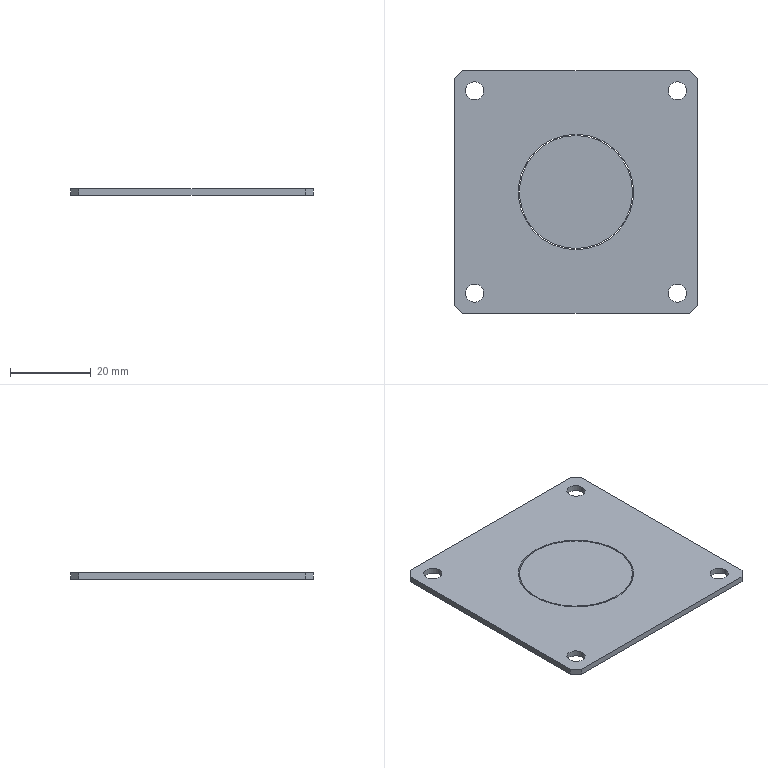Part | STEP file | 接头6 | 1 solid | 32 faces | box 60 x 60 x 1.5 mm | volume 5253 mm3 | cylinder 16 | plane 16 | commonest cylinder face diameters 4.5 x8 27.9 x4 28.5 x4